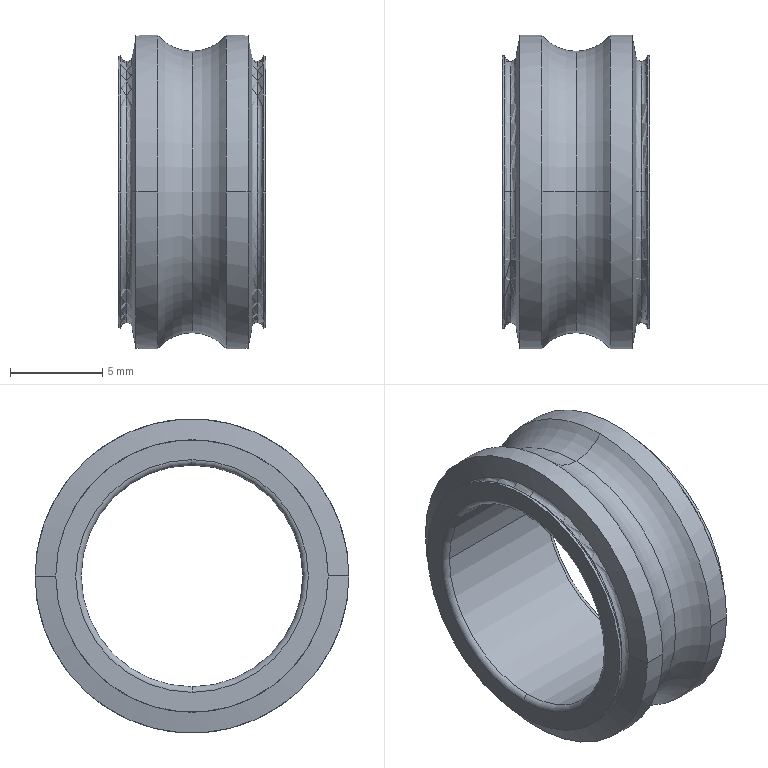Part | SolidWorks | features BaseBody 1 | 1 solid | 32 faces | box 8 x 17 x 17 mm | volume 683.161 mm3 | torus 16 | cylinder 10 | cone 4 | plane 2 | commonest cylinder face diameters 14.75 x4 17 x4 12 x2
STEP:
#1=CARTESIAN_POINT('',(5.849,8.5,0.));
#2=VERTEX_POINT('',#1);
#3=CARTESIAN_POINT('',(7.037,8.5,0.));
#4=VERTEX_POINT('',#3);
#5=CARTESIAN_POINT('',(6.443,8.5,0.));
#6=DIRECTION('',(1.,0.,0.));
#7=VECTOR('',#6,1000.);
#8=LINE('',#5,#7);
#9=EDGE_CURVE('',#2,#4,#8,.T.);
#10=ORIENTED_EDGE('',*,*,#9,.T.);
#11=CARTESIAN_POINT('',(7.037,-8.5,0.));
#12=VERTEX_POINT('',#11);
#13=CARTESIAN_POINT('',(7.037,0.,0.));
#14=DIRECTION('',(1.,0.,0.));
#15=DIRECTION('',(0.,1.,0.));
#16=AXIS2_PLACEMENT_3D('',#13,#14,#15);
#17=CIRCLE('',#16,8.5);
#18=EDGE_CURVE('',#12,#4,#17,.T.);
#19=ORIENTED_EDGE('',*,*,#18,.F.);
#20=CARTESIAN_POINT('',(5.849,-8.5,0.));
#21=VERTEX_POINT('',#20);
#22=CARTESIAN_POINT('',(6.443,-8.5,0.));
#23=DIRECTION('',(-1.,0.,0.));
#24=VECTOR('',#23,1000.);
#25=LINE('',#22,#24);
#26=EDGE_CURVE('',#12,#21,#25,.T.);
#27=ORIENTED_EDGE('',*,*,#26,.T.);
#28=CARTESIAN_POINT('',(5.849,0.,-8.5));
#29=VERTEX_POINT('',#28);
#30=CARTESIAN_POINT('',(5.849,0.,0.));
#31=DIRECTION('',(1.,0.,0.));
#32=DIRECTION('',(0.,1.,0.));
#33=AXIS2_PLACEMENT_3D('',#30,#31,#32);
#34=CIRCLE('',#33,8.5);
#35=EDGE_CURVE('',#21,#29,#34,.T.);
#36=ORIENTED_EDGE('',*,*,#35,.T.);
#37=CARTESIAN_POINT('',(5.849,0.,0.));
#38=DIRECTION('',(1.,0.,0.));
#39=DIRECTION('',(0.,1.,0.));
#40=AXIS2_PLACEMENT_3D('',#37,#38,#39);
#41=CIRCLE('',#40,8.5);
#42=EDGE_CURVE('',#29,#2,#41,.T.);
#43=ORIENTED_EDGE('',*,*,#42,.T.);
#44=EDGE_LOOP('',(#10,#19,#27,#36,#43));
#45=FACE_OUTER_BOUND('',#44,.T.);
#46=CARTESIAN_POINT('',(6.443,0.,0.));
#47=DIRECTION('',(1.,0.,0.));
#48=DIRECTION('',(0.,1.,0.));
#49=AXIS2_PLACEMENT_3D('',#46,#47,#48);
#50=CYLINDRICAL_SURFACE('',#49,8.5);
#51=ADVANCED_FACE('',(#45),#50,.T.);
#52=CARTESIAN_POINT('',(4.,0.,7.619));
#53=VERTEX_POINT('',#52);
#54=CARTESIAN_POINT('',(4.,0.,-7.619));
#55=VERTEX_POINT('',#54);
#56=CARTESIAN_POINT('',(4.,0.,0.));
#57=DIRECTION('',(-1.,0.,0.));
#58=DIRECTION('',(0.,0.,1.));
#59=AXIS2_PLACEMENT_3D('',#56,#57,#58);
#60=CIRCLE('',#59,7.619);
#61=EDGE_CURVE('',#53,#55,#60,.T.);
#62=ORIENTED_EDGE('',*,*,#61,.T.);
#63=CARTESIAN_POINT('',(2.151,0.,-8.5));
#64=VERTEX_POINT('',#63);
#65=CARTESIAN_POINT('',(4.,0.,-10.));
#66=DIRECTION('',(0.,-1.,0.));
#67=DIRECTION('',(0.,0.,-1.));
#68=AXIS2_PLACEMENT_3D('',#65,#66,#67);
#69=CIRCLE('',#68,2.381);
#70=EDGE_CURVE('',#55,#64,#69,.T.);
#71=ORIENTED_EDGE('',*,*,#70,.T.);
#72=CARTESIAN_POINT('',(2.151,8.5,0.));
#73=VERTEX_POINT('',#72);
#74=CARTESIAN_POINT('',(2.151,0.,0.));
#75=DIRECTION('',(1.,0.,0.));
#76=DIRECTION('',(0.,1.,0.));
#77=AXIS2_PLACEMENT_3D('',#74,#75,#76);
#78=CIRCLE('',#77,8.5);
#79=EDGE_CURVE('',#64,#73,#78,.T.);
#80=ORIENTED_EDGE('',*,*,#79,.T.);
#81=CARTESIAN_POINT('',(2.151,0.,8.5));
#82=VERTEX_POINT('',#81);
#83=CARTESIAN_POINT('',(2.151,0.,0.));
#84=DIRECTION('',(1.,0.,0.));
#85=DIRECTION('',(0.,1.,0.));
#86=AXIS2_PLACEMENT_3D('',#83,#84,#85);
#87=CIRCLE('',#86,8.5);
#88=EDGE_CURVE('',#73,#82,#87,.T.);
#89=ORIENTED_EDGE('',*,*,#88,.T.);
#90=CARTESIAN_POINT('',(4.,0.,10.));
#91=DIRECTION('',(0.,-1.,0.));
#92=DIRECTION('',(0.,0.,1.));
#93=AXIS2_PLACEMENT_3D('',#90,#91,#92);
#94=CIRCLE('',#93,2.381);
#95=EDGE_CURVE('',#82,#53,#94,.T.);
#96=ORIENTED_EDGE('',*,*,#95,.T.);
#97=EDGE_LOOP('',(#62,#71,#80,#89,#96));
#98=FACE_OUTER_BOUND('',#97,.T.);
#99=CARTESIAN_POINT('',(4.,0.,0.));
#100=DIRECTION('',(1.,0.,0.));
#101=DIRECTION('',(0.,0.,-1.));
#102=AXIS2_PLACEMENT_3D('',#99,#100,#101);
#103=TOROIDAL_SURFACE('',#102,10.,2.381);
#104=ADVANCED_FACE('',(#98),#103,.F.);
#105=CARTESIAN_POINT('',(0.9631,8.5,0.));
#106=VERTEX_POINT('',#105);
#107=CARTESIAN_POINT('',(1.557,8.5,0.));
#108=DIRECTION('',(1.,0.,0.));
#109=VECTOR('',#108,1000.);
#110=LINE('',#107,#109);
#111=EDGE_CURVE('',#106,#73,#110,.T.);
#112=ORIENTED_EDGE('',*,*,#111,.T.);
#113=ORIENTED_EDGE('',*,*,#79,.F.);
#114=CARTESIAN_POINT('',(2.151,-8.5,0.));
#115=VERTEX_POINT('',#114);
#116=CARTESIAN_POINT('',(2.151,0.,0.));
#117=DIRECTION('',(1.,0.,0.));
#118=DIRECTION('',(0.,1.,0.));
#119=AXIS2_PLACEMENT_3D('',#116,#117,#118);
#120=CIRCLE('',#119,8.5);
#121=EDGE_CURVE('',#115,#64,#120,.T.);
#122=ORIENTED_EDGE('',*,*,#121,.F.);
#123=CARTESIAN_POINT('',(0.9631,-8.5,0.));
#124=VERTEX_POINT('',#123);
#125=CARTESIAN_POINT('',(1.557,-8.5,0.));
#126=DIRECTION('',(-1.,0.,0.));
#127=VECTOR('',#126,1000.);
#128=LINE('',#125,#127);
#129=EDGE_CURVE('',#115,#124,#128,.T.);
#130=ORIENTED_EDGE('',*,*,#129,.T.);
#131=CARTESIAN_POINT('',(0.9631,0.,0.));
#132=DIRECTION('',(1.,0.,0.));
#133=DIRECTION('',(0.,1.,0.));
#134=AXIS2_PLACEMENT_3D('',#131,#132,#133);
#135=CIRCLE('',#134,8.5);
#136=EDGE_CURVE('',#124,#106,#135,.T.);
#137=ORIENTED_EDGE('',*,*,#136,.T.);
#138=EDGE_LOOP('',(#112,#113,#122,#130,#137));
#139=FACE_OUTER_BOUND('',#138,.T.);
#140=CARTESIAN_POINT('',(1.557,0.,0.));
#141=DIRECTION('',(1.,0.,0.));
#142=DIRECTION('',(0.,1.,0.));
#143=AXIS2_PLACEMENT_3D('',#140,#141,#142);
#144=CYLINDRICAL_SURFACE('',#143,8.5);
#145=ADVANCED_FACE('',(#139),#144,.T.);
#146=CARTESIAN_POINT('',(0.7554,7.322,0.));
#147=VERTEX_POINT('',#146);
#148=CARTESIAN_POINT('',(0.8592,7.911,0.));
#149=DIRECTION('',(0.1736,0.9848,0.));
#150=VECTOR('',#149,1000.);
#151=LINE('',#148,#150);
#152=EDGE_CURVE('',#147,#106,#151,.T.);
#153=ORIENTED_EDGE('',*,*,#152,.T.);
#154=ORIENTED_EDGE('',*,*,#136,.F.);
#155=CARTESIAN_POINT('',(0.7554,-7.322,0.));
#156=VERTEX_POINT('',#155);
#157=CARTESIAN_POINT('',(0.8592,-7.911,0.));
#158=DIRECTION('',(-0.1736,0.9848,0.));
#159=VECTOR('',#158,1000.);
#160=LINE('',#157,#159);
#161=EDGE_CURVE('',#124,#156,#160,.T.);
#162=ORIENTED_EDGE('',*,*,#161,.T.);
#163=CARTESIAN_POINT('',(0.7554,0.,-7.322));
#164=VERTEX_POINT('',#163);
#165=CARTESIAN_POINT('',(0.7554,0.,0.));
#166=DIRECTION('',(1.,0.,0.));
#167=DIRECTION('',(0.,1.,0.));
#168=AXIS2_PLACEMENT_3D('',#165,#166,#167);
#169=CIRCLE('',#168,7.322);
#170=EDGE_CURVE('',#156,#164,#169,.T.);
#171=ORIENTED_EDGE('',*,*,#170,.T.);
#172=CARTESIAN_POINT('',(0.7554,0.,0.));
#173=DIRECTION('',(1.,0.,0.));
#174=DIRECTION('',(0.,1.,0.));
#175=AXIS2_PLACEMENT_3D('',#172,#173,#174);
#176=CIRCLE('',#175,7.322);
#177=EDGE_CURVE('',#164,#147,#176,.T.);
#178=ORIENTED_EDGE('',*,*,#177,.T.);
#179=EDGE_LOOP('',(#153,#154,#162,#171,#178));
#180=FACE_OUTER_BOUND('',#179,.T.);
#181=CARTESIAN_POINT('',(0.8592,0.,0.));
#182=DIRECTION('',(1.,0.,0.));
#183=DIRECTION('',(0.,1.,0.));
#184=AXIS2_PLACEMENT_3D('',#181,#182,#183);
#185=CONICAL_SURFACE('',#184,7.911,1.396);
#186=ADVANCED_FACE('',(#180),#185,.T.);
#187=CARTESIAN_POINT('',(0.456,0.,7.071));
#188=VERTEX_POINT('',#187);
#189=CARTESIAN_POINT('',(0.456,0.,-7.071));
#190=VERTEX_POINT('',#189);
#191=CARTESIAN_POINT('',(0.456,0.,0.));
#192=DIRECTION('',(-1.,0.,0.));
#193=DIRECTION('',(0.,0.,1.));
#194=AXIS2_PLACEMENT_3D('',#191,#192,#193);
#195=CIRCLE('',#194,7.071);
#196=EDGE_CURVE('',#188,#190,#195,.T.);
#197=ORIENTED_EDGE('',*,*,#196,.T.);
#198=CARTESIAN_POINT('',(0.152,0.,-7.375));
#199=VERTEX_POINT('',#198);
#200=CARTESIAN_POINT('',(0.456,0.,-7.375));
#201=DIRECTION('',(0.,-1.,0.));
#202=DIRECTION('',(0.,0.,-1.));
#203=AXIS2_PLACEMENT_3D('',#200,#201,#202);
#204=CIRCLE('',#203,0.304);
#205=EDGE_CURVE('',#190,#199,#204,.T.);
#206=ORIENTED_EDGE('',*,*,#205,.T.);
#207=CARTESIAN_POINT('',(0.152,7.375,0.));
#208=VERTEX_POINT('',#207);
#209=CARTESIAN_POINT('',(0.152,0.,0.));
#210=DIRECTION('',(1.,0.,0.));
#211=DIRECTION('',(0.,1.,0.));
#212=AXIS2_PLACEMENT_3D('',#209,#210,#211);
#213=CIRCLE('',#212,7.375);
#214=EDGE_CURVE('',#199,#208,#213,.T.);
#215=ORIENTED_EDGE('',*,*,#214,.T.);
#216=CARTESIAN_POINT('',(0.152,0.,7.375));
#217=VERTEX_POINT('',#216);
#218=CARTESIAN_POINT('',(0.152,0.,0.));
#219=DIRECTION('',(1.,0.,0.));
#220=DIRECTION('',(0.,1.,0.));
#221=AXIS2_PLACEMENT_3D('',#218,#219,#220);
#222=CIRCLE('',#221,7.375);
#223=EDGE_CURVE('',#208,#217,#222,.T.);
#224=ORIENTED_EDGE('',*,*,#223,.T.);
#225=CARTESIAN_POINT('',(0.456,0.,7.375));
#226=DIRECTION('',(0.,-1.,0.));
#227=DIRECTION('',(0.,0.,1.));
#228=AXIS2_PLACEMENT_3D('',#225,#226,#227);
#229=CIRCLE('',#228,0.304);
#230=EDGE_CURVE('',#217,#188,#229,.T.);
#231=ORIENTED_EDGE('',*,*,#230,.T.);
#232=EDGE_LOOP('',(#197,#206,#215,#224,#231));
#233=FACE_OUTER_BOUND('',#232,.T.);
#234=CARTESIAN_POINT('',(0.456,0.,0.));
#235=DIRECTION('',(1.,0.,0.));
#236=DIRECTION('',(0.,0.,-1.));
#237=AXIS2_PLACEMENT_3D('',#234,#235,#236);
#238=TOROIDAL_SURFACE('',#237,7.375,0.304);
#239=ADVANCED_FACE('',(#233),#238,.F.);
#240=CARTESIAN_POINT('',(0.,7.375,0.));
#241=VERTEX_POINT('',#240);
#242=CARTESIAN_POINT('',(0.076,7.375,0.));
#243=DIRECTION('',(1.,0.,0.));
#244=VECTOR('',#243,1000.);
#245=LINE('',#242,#244);
#246=EDGE_CURVE('',#241,#208,#245,.T.);
#247=ORIENTED_EDGE('',*,*,#246,.T.);
#248=ORIENTED_EDGE('',*,*,#214,.F.);
#249=CARTESIAN_POINT('',(0.152,-7.375,0.));
#250=VERTEX_POINT('',#249);
#251=CARTESIAN_POINT('',(0.152,0.,0.));
#252=DIRECTION('',(1.,0.,0.));
#253=DIRECTION('',(0.,1.,0.));
#254=AXIS2_PLACEMENT_3D('',#251,#252,#253);
#255=CIRCLE('',#254,7.375);
#256=EDGE_CURVE('',#250,#199,#255,.T.);
#257=ORIENTED_EDGE('',*,*,#256,.F.);
#258=CARTESIAN_POINT('',(0.,-7.375,0.));
#259=VERTEX_POINT('',#258);
#260=CARTESIAN_POINT('',(0.076,-7.375,0.));
#261=DIRECTION('',(-1.,0.,0.));
#262=VECTOR('',#261,1000.);
#263=LINE('',#260,#262);
#264=EDGE_CURVE('',#250,#259,#263,.T.);
#265=ORIENTED_EDGE('',*,*,#264,.T.);
#266=CARTESIAN_POINT('',(0.,0.,0.));
#267=DIRECTION('',(1.,0.,0.));
#268=DIRECTION('',(0.,1.,0.));
#269=AXIS2_PLACEMENT_3D('',#266,#267,#268);
#270=CIRCLE('',#269,7.375);
#271=EDGE_CURVE('',#259,#241,#270,.T.);
#272=ORIENTED_EDGE('',*,*,#271,.T.);
#273=EDGE_LOOP('',(#247,#248,#257,#265,#272));
#274=FACE_OUTER_BOUND('',#273,.T.);
#275=CARTESIAN_POINT('',(0.076,0.,0.));
#276=DIRECTION('',(1.,0.,0.));
#277=DIRECTION('',(0.,1.,0.));
#278=AXIS2_PLACEMENT_3D('',#275,#276,#277);
#279=CYLINDRICAL_SURFACE('',#278,7.375);
#280=ADVANCED_FACE('',(#274),#279,.T.);
#281=CARTESIAN_POINT('',(0.,0.,6.3));
#282=VERTEX_POINT('',#281);
#283=CARTESIAN_POINT('',(0.,0.,-6.3));
#284=VERTEX_POINT('',#283);
#285=CARTESIAN_POINT('',(0.,0.,0.));
#286=DIRECTION('',(1.,0.,0.));
#287=DIRECTION('',(0.,1.,0.));
#288=AXIS2_PLACEMENT_3D('',#285,#286,#287);
#289=CIRCLE('',#288,6.3);
#290=EDGE_CURVE('',#282,#284,#289,.T.);
#291=ORIENTED_EDGE('',*,*,#290,.T.);
#292=CARTESIAN_POINT('',(0.,0.,0.));
#293=DIRECTION('',(1.,0.,0.));
#294=DIRECTION('',(0.,1.,0.));
#295=AXIS2_PLACEMENT_3D('',#292,#293,#294);
#296=CIRCLE('',#295,6.3);
#297=EDGE_CURVE('',#284,#282,#296,.T.);
#298=ORIENTED_EDGE('',*,*,#297,.T.);
#299=EDGE_LOOP('',(#291,#298));
#300=FACE_BOUND('',#299,.T.);
#301=CARTESIAN_POINT('',(0.,0.,0.));
#302=DIRECTION('',(1.,0.,0.));
#303=DIRECTION('',(0.,1.,0.));
#304=AXIS2_PLACEMENT_3D('',#301,#302,#303);
#305=CIRCLE('',#304,7.375);
#306=EDGE_CURVE('',#241,#259,#305,.T.);
#307=ORIENTED_EDGE('',*,*,#306,.F.);
#308=ORIENTED_EDGE('',*,*,#271,.F.);
#309=EDGE_LOOP('',(#307,#308));
#310=FACE_OUTER_BOUND('',#309,.T.);
#311=CARTESIAN_POINT('',(0.,6.837,0.));
#312=DIRECTION('',(-1.,0.,0.));
#313=DIRECTION('',(0.,0.,1.));
#314=AXIS2_PLACEMENT_3D('',#311,#312,#313);
#315=PLANE('',#314);
#316=ADVANCED_FACE('',(#300,#310),#315,.T.);
#317=CARTESIAN_POINT('',(0.3,0.,-6.));
#318=VERTEX_POINT('',#317);
#319=CARTESIAN_POINT('',(0.3,0.,-6.3));
#320=DIRECTION('',(0.,-1.,0.));
#321=DIRECTION('',(0.,0.,-1.));
#322=AXIS2_PLACEMENT_3D('',#319,#320,#321);
#323=CIRCLE('',#322,0.3);
#324=EDGE_CURVE('',#318,#284,#323,.T.);
#325=ORIENTED_EDGE('',*,*,#324,.T.);
#326=ORIENTED_EDGE('',*,*,#290,.F.);
#327=CARTESIAN_POINT('',(0.3,0.,6.));
#328=VERTEX_POINT('',#327);
#329=CARTESIAN_POINT('',(0.3,0.,6.3));
#330=DIRECTION('',(0.,-1.,0.));
#331=DIRECTION('',(0.,0.,1.));
#332=AXIS2_PLACEMENT_3D('',#329,#330,#331);
#333=CIRCLE('',#332,0.3);
#334=EDGE_CURVE('',#282,#328,#333,.T.);
#335=ORIENTED_EDGE('',*,*,#334,.T.);
#336=CARTESIAN_POINT('',(0.3,-6.,0.));
#337=VERTEX_POINT('',#336);
#338=CARTESIAN_POINT('',(0.3,0.,0.));
#339=DIRECTION('',(1.,0.,0.));
#340=DIRECTION('',(0.,1.,0.));
#341=AXIS2_PLACEMENT_3D('',#338,#339,#340);
#342=CIRCLE('',#341,6.);
#343=EDGE_CURVE('',#328,#337,#342,.T.);
#344=ORIENTED_EDGE('',*,*,#343,.T.);
#345=CARTESIAN_POINT('',(0.3,0.,0.));
#346=DIRECTION('',(1.,0.,0.));
#347=DIRECTION('',(0.,1.,0.));
#348=AXIS2_PLACEMENT_3D('',#345,#346,#347);
#349=CIRCLE('',#348,6.);
#350=EDGE_CURVE('',#337,#318,#349,.T.);
#351=ORIENTED_EDGE('',*,*,#350,.T.);
#352=EDGE_LOOP('',(#325,#326,#335,#344,#351));
#353=FACE_OUTER_BOUND('',#352,.T.);
#354=CARTESIAN_POINT('',(0.3,0.,0.));
#355=DIRECTION('',(1.,0.,0.));
#356=DIRECTION('',(0.,0.,-1.));
#357=AXIS2_PLACEMENT_3D('',#354,#355,#356);
#358=TOROIDAL_SURFACE('',#357,6.3,0.3);
#359=ADVANCED_FACE('',(#353),#358,.T.);
#360=CARTESIAN_POINT('',(0.3,6.,0.));
#361=VERTEX_POINT('',#360);
#362=CARTESIAN_POINT('',(7.7,6.,0.));
#363=VERTEX_POINT('',#362);
#364=CARTESIAN_POINT('',(4.,6.,0.));
#365=DIRECTION('',(1.,0.,0.));
#366=VECTOR('',#365,1000.);
#367=LINE('',#364,#366);
#368=EDGE_CURVE('',#361,#363,#367,.T.);
#369=ORIENTED_EDGE('',*,*,#368,.T.);
#370=CARTESIAN_POINT('',(7.7,0.,6.));
#371=VERTEX_POINT('',#370);
#372=CARTESIAN_POINT('',(7.7,0.,0.));
#373=DIRECTION('',(1.,0.,0.));
#374=DIRECTION('',(0.,1.,0.));
#375=AXIS2_PLACEMENT_3D('',#372,#373,#374);
#376=CIRCLE('',#375,6.);
#377=EDGE_CURVE('',#363,#371,#376,.T.);
#378=ORIENTED_EDGE('',*,*,#377,.T.);
#379=CARTESIAN_POINT('',(7.7,-6.,0.));
#380=VERTEX_POINT('',#379);
#381=CARTESIAN_POINT('',(7.7,0.,0.));
#382=DIRECTION('',(1.,0.,0.));
#383=DIRECTION('',(0.,1.,0.));
#384=AXIS2_PLACEMENT_3D('',#381,#382,#383);
#385=CIRCLE('',#384,6.);
#386=EDGE_CURVE('',#371,#380,#385,.T.);
#387=ORIENTED_EDGE('',*,*,#386,.T.);
#388=CARTESIAN_POINT('',(4.,-6.,0.));
#389=DIRECTION('',(-1.,0.,0.));
#390=VECTOR('',#389,1000.);
#391=LINE('',#388,#390);
#392=EDGE_CURVE('',#380,#337,#391,.T.);
#393=ORIENTED_EDGE('',*,*,#392,.T.);
#394=ORIENTED_EDGE('',*,*,#343,.F.);
#395=CARTESIAN_POINT('',(0.3,0.,0.));
#396=DIRECTION('',(1.,0.,0.));
#397=DIRECTION('',(0.,1.,0.));
#398=AXIS2_PLACEMENT_3D('',#395,#396,#397);
#399=CIRCLE('',#398,6.);
#400=EDGE_CURVE('',#361,#328,#399,.T.);
#401=ORIENTED_EDGE('',*,*,#400,.F.);
#402=EDGE_LOOP('',(#369,#378,#387,#393,#394,#401));
#403=FACE_OUTER_BOUND('',#402,.T.);
#404=CARTESIAN_POINT('',(4.,0.,0.));
#405=DIRECTION('',(1.,0.,0.));
#406=DIRECTION('',(0.,1.,0.));
#407=AXIS2_PLACEMENT_3D('',#404,#405,#406);
#408=CYLINDRICAL_SURFACE('',#407,6.);
#409=ADVANCED_FACE('',(#403),#408,.F.);
#410=CARTESIAN_POINT('',(8.,0.,-6.3));
#411=VERTEX_POINT('',#410);
#412=CARTESIAN_POINT('',(7.7,0.,-6.));
#413=VERTEX_POINT('',#412);
#414=CARTESIAN_POINT('',(7.7,0.,-6.3));
#415=DIRECTION('',(0.,-1.,0.));
#416=DIRECTION('',(0.,0.,-1.));
#417=AXIS2_PLACEMENT_3D('',#414,#415,#416);
#418=CIRCLE('',#417,0.3);
#419=EDGE_CURVE('',#411,#413,#418,.T.);
#420=ORIENTED_EDGE('',*,*,#419,.T.);
#421=CARTESIAN_POINT('',(7.7,0.,0.));
#422=DIRECTION('',(1.,0.,0.));
#423=DIRECTION('',(0.,1.,0.));
#424=AXIS2_PLACEMENT_3D('',#421,#422,#423);
#425=CIRCLE('',#424,6.);
#426=EDGE_CURVE('',#380,#413,#425,.T.);
#427=ORIENTED_EDGE('',*,*,#426,.F.);
#428=ORIENTED_EDGE('',*,*,#386,.F.);
#429=CARTESIAN_POINT('',(8.,0.,6.3));
#430=VERTEX_POINT('',#429);
#431=CARTESIAN_POINT('',(7.7,0.,6.3));
#432=DIRECTION('',(0.,-1.,0.));
#433=DIRECTION('',(0.,0.,1.));
#434=AXIS2_PLACEMENT_3D('',#431,#432,#433);
#435=CIRCLE('',#434,0.3);
#436=EDGE_CURVE('',#371,#430,#435,.T.);
#437=ORIENTED_EDGE('',*,*,#436,.T.);
#438=CARTESIAN_POINT('',(8.,0.,0.));
#439=DIRECTION('',(1.,0.,0.));
#440=DIRECTION('',(0.,1.,0.));
#441=AXIS2_PLACEMENT_3D('',#438,#439,#440);
#442=CIRCLE('',#441,6.3);
#443=EDGE_CURVE('',#430,#411,#442,.T.);
#444=ORIENTED_EDGE('',*,*,#443,.T.);
#445=EDGE_LOOP('',(#420,#427,#428,#437,#444));
#446=FACE_OUTER_BOUND('',#445,.T.);
#447=CARTESIAN_POINT('',(7.7,0.,0.));
#448=DIRECTION('',(1.,0.,0.));
#449=DIRECTION('',(0.,0.,-1.));
#450=AXIS2_PLACEMENT_3D('',#447,#448,#449);
#451=TOROIDAL_SURFACE('',#450,6.3,0.3);
#452=ADVANCED_FACE('',(#446),#451,.T.);
#453=CARTESIAN_POINT('',(8.,0.,0.));
#454=DIRECTION('',(1.,0.,0.));
#455=DIRECTION('',(0.,1.,0.));
#456=AXIS2_PLACEMENT_3D('',#453,#454,#455);
#457=CIRCLE('',#456,6.3);
#458=EDGE_CURVE('',#411,#430,#457,.T.);
#459=ORIENTED_EDGE('',*,*,#458,.F.);
#460=ORIENTED_EDGE('',*,*,#443,.F.);
#461=EDGE_LOOP('',(#459,#460));
#462=FACE_BOUND('',#461,.T.);
#463=CARTESIAN_POINT('',(8.,7.375,0.));
#464=VERTEX_POINT('',#463);
#465=CARTESIAN_POINT('',(8.,-7.375,0.));
#466=VERTEX_POINT('',#465);
#467=CARTESIAN_POINT('',(8.,0.,0.));
#468=DIRECTION('',(1.,0.,0.));
#469=DIRECTION('',(0.,1.,0.));
#470=AXIS2_PLACEMENT_3D('',#467,#468,#469);
#471=CIRCLE('',#470,7.375);
#472=EDGE_CURVE('',#464,#466,#471,.T.);
#473=ORIENTED_EDGE('',*,*,#472,.T.);
#474=CARTESIAN_POINT('',(8.,0.,0.));
#475=DIRECTION('',(1.,0.,0.));
#476=DIRECTION('',(0.,1.,0.));
#477=AXIS2_PLACEMENT_3D('',#474,#475,#476);
#478=CIRCLE('',#477,7.375);
#479=EDGE_CURVE('',#466,#464,#478,.T.);
#480=ORIENTED_EDGE('',*,*,#479,.T.);
#481=EDGE_LOOP('',(#473,#480));
#482=FACE_OUTER_BOUND('',#481,.T.);
#483=CARTESIAN_POINT('',(8.,6.837,0.));
#484=DIRECTION('',(1.,0.,0.));
#485=DIRECTION('',(0.,1.,0.));
#486=AXIS2_PLACEMENT_3D('',#483,#484,#485);
#487=PLANE('',#486);
#488=ADVANCED_FACE('',(#462,#482),#487,.T.);
#489=CARTESIAN_POINT('',(7.848,7.375,0.));
#490=VERTEX_POINT('',#489);
#491=CARTESIAN_POINT('',(7.924,7.375,0.));
#492=DIRECTION('',(1.,0.,0.));
#493=VECTOR('',#492,1000.);
#494=LINE('',#491,#493);
#495=EDGE_CURVE('',#490,#464,#494,.T.);
#496=ORIENTED_EDGE('',*,*,#495,.T.);
#497=ORIENTED_EDGE('',*,*,#479,.F.);
#498=CARTESIAN_POINT('',(7.848,-7.375,0.));
#499=VERTEX_POINT('',#498);
#500=CARTESIAN_POINT('',(7.924,-7.375,0.));
#501=DIRECTION('',(-1.,0.,0.));
#502=VECTOR('',#501,1000.);
#503=LINE('',#500,#502);
#504=EDGE_CURVE('',#466,#499,#503,.T.);
#505=ORIENTED_EDGE('',*,*,#504,.T.);
#506=CARTESIAN_POINT('',(7.848,0.,-7.375));
#507=VERTEX_POINT('',#506);
#508=CARTESIAN_POINT('',(7.848,0.,0.));
#509=DIRECTION('',(1.,0.,0.));
#510=DIRECTION('',(0.,1.,0.));
#511=AXIS2_PLACEMENT_3D('',#508,#509,#510);
#512=CIRCLE('',#511,7.375);
#513=EDGE_CURVE('',#499,#507,#512,.T.);
#514=ORIENTED_EDGE('',*,*,#513,.T.);
#515=CARTESIAN_POINT('',(7.848,0.,0.));
#516=DIRECTION('',(1.,0.,0.));
#517=DIRECTION('',(0.,1.,0.));
#518=AXIS2_PLACEMENT_3D('',#515,#516,#517);
#519=CIRCLE('',#518,7.375);
#520=EDGE_CURVE('',#507,#490,#519,.T.);
#521=ORIENTED_EDGE('',*,*,#520,.T.);
#522=EDGE_LOOP('',(#496,#497,#505,#514,#521));
#523=FACE_OUTER_BOUND('',#522,.T.);
#524=CARTESIAN_POINT('',(7.924,0.,0.));
#525=DIRECTION('',(1.,0.,0.));
#526=DIRECTION('',(0.,1.,0.));
#527=AXIS2_PLACEMENT_3D('',#524,#525,#526);
#528=CYLINDRICAL_SURFACE('',#527,7.375);
#529=ADVANCED_FACE('',(#523),#528,.T.);
#530=CARTESIAN_POINT('',(7.544,0.,7.071));
#531=VERTEX_POINT('',#530);
#532=CARTESIAN_POINT('',(7.544,0.,-7.071));
#533=VERTEX_POINT('',#532);
#534=CARTESIAN_POINT('',(7.544,0.,0.));
#535=DIRECTION('',(-1.,0.,0.));
#536=DIRECTION('',(0.,0.,1.));
#537=AXIS2_PLACEMENT_3D('',#534,#535,#536);
#538=CIRCLE('',#537,7.071);
#539=EDGE_CURVE('',#531,#533,#538,.T.);
#540=ORIENTED_EDGE('',*,*,#539,.T.);
#541=CARTESIAN_POINT('',(7.245,0.,-7.322));
#542=VERTEX_POINT('',#541);
#543=CARTESIAN_POINT('',(7.544,0.,-7.375));
#544=DIRECTION('',(0.,-1.,0.));
#545=DIRECTION('',(0.,0.,-1.));
#546=AXIS2_PLACEMENT_3D('',#543,#544,#545);
#547=CIRCLE('',#546,0.304);
#548=EDGE_CURVE('',#533,#542,#547,.T.);
#549=ORIENTED_EDGE('',*,*,#548,.T.);
#550=CARTESIAN_POINT('',(7.245,7.322,0.));
#551=VERTEX_POINT('',#550);
#552=CARTESIAN_POINT('',(7.245,0.,0.));
#553=DIRECTION('',(1.,0.,0.));
#554=DIRECTION('',(0.,1.,0.));
#555=AXIS2_PLACEMENT_3D('',#552,#553,#554);
#556=CIRCLE('',#555,7.322);
#557=EDGE_CURVE('',#542,#551,#556,.T.);
#558=ORIENTED_EDGE('',*,*,#557,.T.);
#559=CARTESIAN_POINT('',(7.245,0.,7.322));
#560=VERTEX_POINT('',#559);
#561=CARTESIAN_POINT('',(7.245,0.,0.));
#562=DIRECTION('',(1.,0.,0.));
#563=DIRECTION('',(0.,1.,0.));
#564=AXIS2_PLACEMENT_3D('',#561,#562,#563);
#565=CIRCLE('',#564,7.322);
#566=EDGE_CURVE('',#551,#560,#565,.T.);
#567=ORIENTED_EDGE('',*,*,#566,.T.);
#568=CARTESIAN_POINT('',(7.544,0.,7.375));
#569=DIRECTION('',(0.,-1.,0.));
#570=DIRECTION('',(0.,0.,1.));
#571=AXIS2_PLACEMENT_3D('',#568,#569,#570);
#572=CIRCLE('',#571,0.304);
#573=EDGE_CURVE('',#560,#531,#572,.T.);
#574=ORIENTED_EDGE('',*,*,#573,.T.);
#575=EDGE_LOOP('',(#540,#549,#558,#567,#574));
#576=FACE_OUTER_BOUND('',#575,.T.);
#577=CARTESIAN_POINT('',(7.544,0.,0.));
#578=DIRECTION('',(1.,0.,0.));
#579=DIRECTION('',(0.,0.,-1.));
#580=AXIS2_PLACEMENT_3D('',#577,#578,#579);
#581=TOROIDAL_SURFACE('',#580,7.375,0.304);
#582=ADVANCED_FACE('',(#576),#581,.F.);
#583=CARTESIAN_POINT('',(7.141,7.911,0.));
#584=DIRECTION('',(0.1736,-0.9848,0.));
#585=VECTOR('',#584,1000.);
#586=LINE('',#583,#585);
#587=EDGE_CURVE('',#4,#551,#586,.T.);
#588=ORIENTED_EDGE('',*,*,#587,.T.);
#589=ORIENTED_EDGE('',*,*,#557,.F.);
#590=CARTESIAN_POINT('',(7.245,-7.322,0.));
#591=VERTEX_POINT('',#590);
#592=CARTESIAN_POINT('',(7.245,0.,0.));
#593=DIRECTION('',(1.,0.,0.));
#594=DIRECTION('',(0.,1.,0.));
#595=AXIS2_PLACEMENT_3D('',#592,#593,#594);
#596=CIRCLE('',#595,7.322);
#597=EDGE_CURVE('',#591,#542,#596,.T.);
#598=ORIENTED_EDGE('',*,*,#597,.F.);
#599=CARTESIAN_POINT('',(7.141,-7.911,0.));
#600=DIRECTION('',(-0.1736,-0.9848,0.));
#601=VECTOR('',#600,1000.);
#602=LINE('',#599,#601);
#603=EDGE_CURVE('',#591,#12,#602,.T.);
#604=ORIENTED_EDGE('',*,*,#603,.T.);
#605=ORIENTED_EDGE('',*,*,#18,.T.);
#606=EDGE_LOOP('',(#588,#589,#598,#604,#605));
#607=FACE_OUTER_BOUND('',#606,.T.);
#608=CARTESIAN_POINT('',(7.141,0.,0.));
#609=DIRECTION('',(-1.,0.,0.));
#610=DIRECTION('',(0.,1.,0.));
#611=AXIS2_PLACEMENT_3D('',#608,#609,#610);
#612=CONICAL_SURFACE('',#611,7.911,1.396);
#613=ADVANCED_FACE('',(#607),#612,.T.);
#614=ORIENTED_EDGE('',*,*,#587,.F.);
#615=CARTESIAN_POINT('',(7.037,0.,0.));
#616=DIRECTION('',(1.,0.,0.));
#617=DIRECTION('',(0.,1.,0.));
#618=AXIS2_PLACEMENT_3D('',#615,#616,#617);
#619=CIRCLE('',#618,8.5);
#620=EDGE_CURVE('',#4,#12,#619,.T.);
#621=ORIENTED_EDGE('',*,*,#620,.T.);
#622=ORIENTED_EDGE('',*,*,#603,.F.);
#623=CARTESIAN_POINT('',(7.245,0.,0.));
#624=DIRECTION('',(1.,0.,0.));
#625=DIRECTION('',(0.,1.,0.));
#626=AXIS2_PLACEMENT_3D('',#623,#624,#625);
#627=CIRCLE('',#626,7.322);
#628=EDGE_CURVE('',#560,#591,#627,.T.);
#629=ORIENTED_EDGE('',*,*,#628,.F.);
#630=ORIENTED_EDGE('',*,*,#566,.F.);
#631=EDGE_LOOP('',(#614,#621,#622,#629,#630));
#632=FACE_OUTER_BOUND('',#631,.T.);
#633=CARTESIAN_POINT('',(7.141,0.,0.));
#634=DIRECTION('',(-1.,0.,0.));
#635=DIRECTION('',(0.,1.,0.));
#636=AXIS2_PLACEMENT_3D('',#633,#634,#635);
#637=CONICAL_SURFACE('',#636,7.911,1.396);
#638=ADVANCED_FACE('',(#632),#637,.T.);
#639=CARTESIAN_POINT('',(7.544,0.,0.));
#640=DIRECTION('',(-1.,0.,0.));
#641=DIRECTION('',(0.,0.,1.));
#642=AXIS2_PLACEMENT_3D('',#639,#640,#641);
#643=CIRCLE('',#642,7.071);
#644=EDGE_CURVE('',#533,#531,#643,.T.);
#645=ORIENTED_EDGE('',*,*,#644,.T.);
#646=ORIENTED_EDGE('',*,*,#573,.F.);
#647=ORIENTED_EDGE('',*,*,#628,.T.);
#648=ORIENTED_EDGE('',*,*,#597,.T.);
#649=ORIENTED_EDGE('',*,*,#548,.F.);
#650=EDGE_LOOP('',(#645,#646,#647,#648,#649));
#651=FACE_OUTER_BOUND('',#650,.T.);
#652=CARTESIAN_POINT('',(7.544,0.,0.));
#653=DIRECTION('',(1.,0.,0.));
#654=DIRECTION('',(0.,0.,-1.));
#655=AXIS2_PLACEMENT_3D('',#652,#653,#654);
#656=TOROIDAL_SURFACE('',#655,7.375,0.304);
#657=ADVANCED_FACE('',(#651),#656,.F.);
#658=ORIENTED_EDGE('',*,*,#495,.F.);
#659=CARTESIAN_POINT('',(7.848,0.,7.375));
#660=VERTEX_POINT('',#659);
#661=CARTESIAN_POINT('',(7.848,0.,0.));
#662=DIRECTION('',(1.,0.,0.));
#663=DIRECTION('',(0.,1.,0.));
#664=AXIS2_PLACEMENT_3D('',#661,#662,#663);
#665=CIRCLE('',#664,7.375);
#666=EDGE_CURVE('',#490,#660,#665,.T.);
#667=ORIENTED_EDGE('',*,*,#666,.T.);
#668=CARTESIAN_POINT('',(7.848,0.,0.));
#669=DIRECTION('',(1.,0.,0.));
#670=DIRECTION('',(0.,1.,0.));
#671=AXIS2_PLACEMENT_3D('',#668,#669,#670);
#672=CIRCLE('',#671,7.375);
#673=EDGE_CURVE('',#660,#499,#672,.T.);
#674=ORIENTED_EDGE('',*,*,#673,.T.);
#675=ORIENTED_EDGE('',*,*,#504,.F.);
#676=ORIENTED_EDGE('',*,*,#472,.F.);
#677=EDGE_LOOP('',(#658,#667,#674,#675,#676));
#678=FACE_OUTER_BOUND('',#677,.T.);
#679=CARTESIAN_POINT('',(7.924,0.,0.));
#680=DIRECTION('',(1.,0.,0.));
#681=DIRECTION('',(0.,1.,0.));
#682=AXIS2_PLACEMENT_3D('',#679,#680,#681);
#683=CYLINDRICAL_SURFACE('',#682,7.375);
#684=ADVANCED_FACE('',(#678),#683,.T.);
#685=ORIENTED_EDGE('',*,*,#419,.F.);
#686=ORIENTED_EDGE('',*,*,#458,.T.);
#687=ORIENTED_EDGE('',*,*,#436,.F.);
#688=ORIENTED_EDGE('',*,*,#377,.F.);
#689=CARTESIAN_POINT('',(7.7,0.,0.));
#690=DIRECTION('',(1.,0.,0.));
#691=DIRECTION('',(0.,1.,0.));
#692=AXIS2_PLACEMENT_3D('',#689,#690,#691);
#693=CIRCLE('',#692,6.);
#694=EDGE_CURVE('',#413,#363,#693,.T.);
#695=ORIENTED_EDGE('',*,*,#694,.F.);
#696=EDGE_LOOP('',(#685,#686,#687,#688,#695));
#697=FACE_OUTER_BOUND('',#696,.T.);
#698=CARTESIAN_POINT('',(7.7,0.,0.));
#699=DIRECTION('',(1.,0.,0.));
#700=DIRECTION('',(0.,0.,-1.));
#701=AXIS2_PLACEMENT_3D('',#698,#699,#700);
#702=TOROIDAL_SURFACE('',#701,6.3,0.3);
#703=ADVANCED_FACE('',(#697),#702,.T.);
#704=ORIENTED_EDGE('',*,*,#368,.F.);
#705=CARTESIAN_POINT('',(0.3,0.,0.));
#706=DIRECTION('',(1.,0.,0.));
#707=DIRECTION('',(0.,1.,0.));
#708=AXIS2_PLACEMENT_3D('',#705,#706,#707);
#709=CIRCLE('',#708,6.);
#710=EDGE_CURVE('',#318,#361,#709,.T.);
#711=ORIENTED_EDGE('',*,*,#710,.F.);
#712=ORIENTED_EDGE('',*,*,#350,.F.);
#713=ORIENTED_EDGE('',*,*,#392,.F.);
#714=ORIENTED_EDGE('',*,*,#426,.T.);
#715=ORIENTED_EDGE('',*,*,#694,.T.);
#716=EDGE_LOOP('',(#704,#711,#712,#713,#714,#715));
#717=FACE_OUTER_BOUND('',#716,.T.);
#718=CARTESIAN_POINT('',(4.,0.,0.));
#719=DIRECTION('',(1.,0.,0.));
#720=DIRECTION('',(0.,1.,0.));
#721=AXIS2_PLACEMENT_3D('',#718,#719,#720);
#722=CYLINDRICAL_SURFACE('',#721,6.);
#723=ADVANCED_FACE('',(#717),#722,.F.);
#724=ORIENTED_EDGE('',*,*,#324,.F.);
#725=ORIENTED_EDGE('',*,*,#710,.T.);
#726=ORIENTED_EDGE('',*,*,#400,.T.);
#727=ORIENTED_EDGE('',*,*,#334,.F.);
#728=ORIENTED_EDGE('',*,*,#297,.F.);
#729=EDGE_LOOP('',(#724,#725,#726,#727,#728));
#730=FACE_OUTER_BOUND('',#729,.T.);
#731=CARTESIAN_POINT('',(0.3,0.,0.));
#732=DIRECTION('',(1.,0.,0.));
#733=DIRECTION('',(0.,0.,-1.));
#734=AXIS2_PLACEMENT_3D('',#731,#732,#733);
#735=TOROIDAL_SURFACE('',#734,6.3,0.3);
#736=ADVANCED_FACE('',(#730),#735,.T.);
#737=ORIENTED_EDGE('',*,*,#246,.F.);
#738=ORIENTED_EDGE('',*,*,#306,.T.);
#739=ORIENTED_EDGE('',*,*,#264,.F.);
#740=CARTESIAN_POINT('',(0.152,0.,0.));
#741=DIRECTION('',(1.,0.,0.));
#742=DIRECTION('',(0.,1.,0.));
#743=AXIS2_PLACEMENT_3D('',#740,#741,#742);
#744=CIRCLE('',#743,7.375);
#745=EDGE_CURVE('',#217,#250,#744,.T.);
#746=ORIENTED_EDGE('',*,*,#745,.F.);
#747=ORIENTED_EDGE('',*,*,#223,.F.);
#748=EDGE_LOOP('',(#737,#738,#739,#746,#747));
#749=FACE_OUTER_BOUND('',#748,.T.);
#750=CARTESIAN_POINT('',(0.076,0.,0.));
#751=DIRECTION('',(1.,0.,0.));
#752=DIRECTION('',(0.,1.,0.));
#753=AXIS2_PLACEMENT_3D('',#750,#751,#752);
#754=CYLINDRICAL_SURFACE('',#753,7.375);
#755=ADVANCED_FACE('',(#749),#754,.T.);
#756=CARTESIAN_POINT('',(0.456,0.,0.));
#757=DIRECTION('',(-1.,0.,0.));
#758=DIRECTION('',(0.,0.,1.));
#759=AXIS2_PLACEMENT_3D('',#756,#757,#758);
#760=CIRCLE('',#759,7.071);
#761=EDGE_CURVE('',#190,#188,#760,.T.);
#762=ORIENTED_EDGE('',*,*,#761,.T.);
#763=ORIENTED_EDGE('',*,*,#230,.F.);
#764=ORIENTED_EDGE('',*,*,#745,.T.);
#765=ORIENTED_EDGE('',*,*,#256,.T.);
#766=ORIENTED_EDGE('',*,*,#205,.F.);
#767=EDGE_LOOP('',(#762,#763,#764,#765,#766));
#768=FACE_OUTER_BOUND('',#767,.T.);
#769=CARTESIAN_POINT('',(0.456,0.,0.));
#770=DIRECTION('',(1.,0.,0.));
#771=DIRECTION('',(0.,0.,-1.));
#772=AXIS2_PLACEMENT_3D('',#769,#770,#771);
#773=TOROIDAL_SURFACE('',#772,7.375,0.304);
#774=ADVANCED_FACE('',(#768),#773,.F.);
#775=ORIENTED_EDGE('',*,*,#152,.F.);
#776=CARTESIAN_POINT('',(0.7554,0.,7.322));
#777=VERTEX_POINT('',#776);
#778=CARTESIAN_POINT('',(0.7554,0.,0.));
#779=DIRECTION('',(1.,0.,0.));
#780=DIRECTION('',(0.,1.,0.));
#781=AXIS2_PLACEMENT_3D('',#778,#779,#780);
#782=CIRCLE('',#781,7.322);
#783=EDGE_CURVE('',#147,#777,#782,.T.);
#784=ORIENTED_EDGE('',*,*,#783,.T.);
#785=CARTESIAN_POINT('',(0.7554,0.,0.));
#786=DIRECTION('',(1.,0.,0.));
#787=DIRECTION('',(0.,1.,0.));
#788=AXIS2_PLACEMENT_3D('',#785,#786,#787);
#789=CIRCLE('',#788,7.322);
#790=EDGE_CURVE('',#777,#156,#789,.T.);
#791=ORIENTED_EDGE('',*,*,#790,.T.);
#792=ORIENTED_EDGE('',*,*,#161,.F.);
#793=CARTESIAN_POINT('',(0.9631,0.,0.));
#794=DIRECTION('',(1.,0.,0.));
#795=DIRECTION('',(0.,1.,0.));
#796=AXIS2_PLACEMENT_3D('',#793,#794,#795);
#797=CIRCLE('',#796,8.5);
#798=EDGE_CURVE('',#106,#124,#797,.T.);
#799=ORIENTED_EDGE('',*,*,#798,.F.);
#800=EDGE_LOOP('',(#775,#784,#791,#792,#799));
#801=FACE_OUTER_BOUND('',#800,.T.);
#802=CARTESIAN_POINT('',(0.8592,0.,0.));
#803=DIRECTION('',(1.,0.,0.));
#804=DIRECTION('',(0.,1.,0.));
#805=AXIS2_PLACEMENT_3D('',#802,#803,#804);
#806=CONICAL_SURFACE('',#805,7.911,1.396);
#807=ADVANCED_FACE('',(#801),#806,.T.);
#808=ORIENTED_EDGE('',*,*,#111,.F.);
#809=ORIENTED_EDGE('',*,*,#798,.T.);
#810=ORIENTED_EDGE('',*,*,#129,.F.);
#811=CARTESIAN_POINT('',(2.151,0.,0.));
#812=DIRECTION('',(1.,0.,0.));
#813=DIRECTION('',(0.,1.,0.));
#814=AXIS2_PLACEMENT_3D('',#811,#812,#813);
#815=CIRCLE('',#814,8.5);
#816=EDGE_CURVE('',#82,#115,#815,.T.);
#817=ORIENTED_EDGE('',*,*,#816,.F.);
#818=ORIENTED_EDGE('',*,*,#88,.F.);
#819=EDGE_LOOP('',(#808,#809,#810,#817,#818));
#820=FACE_OUTER_BOUND('',#819,.T.);
#821=CARTESIAN_POINT('',(1.557,0.,0.));
#822=DIRECTION('',(1.,0.,0.));
#823=DIRECTION('',(0.,1.,0.));
#824=AXIS2_PLACEMENT_3D('',#821,#822,#823);
#825=CYLINDRICAL_SURFACE('',#824,8.5);
#826=ADVANCED_FACE('',(#820),#825,.T.);
#827=CARTESIAN_POINT('',(4.,0.,0.));
#828=DIRECTION('',(-1.,0.,0.));
#829=DIRECTION('',(0.,0.,1.));
#830=AXIS2_PLACEMENT_3D('',#827,#828,#829);
#831=CIRCLE('',#830,7.619);
#832=EDGE_CURVE('',#55,#53,#831,.T.);
#833=ORIENTED_EDGE('',*,*,#832,.T.);
#834=ORIENTED_EDGE('',*,*,#95,.F.);
#835=ORIENTED_EDGE('',*,*,#816,.T.);
#836=ORIENTED_EDGE('',*,*,#121,.T.);
#837=ORIENTED_EDGE('',*,*,#70,.F.);
#838=EDGE_LOOP('',(#833,#834,#835,#836,#837));
#839=FACE_OUTER_BOUND('',#838,.T.);
#840=CARTESIAN_POINT('',(4.,0.,0.));
#841=DIRECTION('',(1.,0.,0.));
#842=DIRECTION('',(0.,0.,-1.));
#843=AXIS2_PLACEMENT_3D('',#840,#841,#842);
#844=TOROIDAL_SURFACE('',#843,10.,2.381);
#845=ADVANCED_FACE('',(#839),#844,.F.);
#846=ORIENTED_EDGE('',*,*,#9,.F.);
#847=CARTESIAN_POINT('',(5.849,0.,8.5));
#848=VERTEX_POINT('',#847);
#849=CARTESIAN_POINT('',(5.849,0.,0.));
#850=DIRECTION('',(1.,0.,0.));
#851=DIRECTION('',(0.,1.,0.));
#852=AXIS2_PLACEMENT_3D('',#849,#850,#851);
#853=CIRCLE('',#852,8.5);
#854=EDGE_CURVE('',#2,#848,#853,.T.);
#855=ORIENTED_EDGE('',*,*,#854,.T.);
#856=CARTESIAN_POINT('',(5.849,0.,0.));
#857=DIRECTION('',(1.,0.,0.));
#858=DIRECTION('',(0.,1.,0.));
#859=AXIS2_PLACEMENT_3D('',#856,#857,#858);
#860=CIRCLE('',#859,8.5);
#861=EDGE_CURVE('',#848,#21,#860,.T.);
#862=ORIENTED_EDGE('',*,*,#861,.T.);
#863=ORIENTED_EDGE('',*,*,#26,.F.);
#864=ORIENTED_EDGE('',*,*,#620,.F.);
#865=EDGE_LOOP('',(#846,#855,#862,#863,#864));
#866=FACE_OUTER_BOUND('',#865,.T.);
#867=CARTESIAN_POINT('',(6.443,0.,0.));
#868=DIRECTION('',(1.,0.,0.));
#869=DIRECTION('',(0.,1.,0.));
#870=AXIS2_PLACEMENT_3D('',#867,#868,#869);
#871=CYLINDRICAL_SURFACE('',#870,8.5);
#872=ADVANCED_FACE('',(#866),#871,.T.);
#873=ORIENTED_EDGE('',*,*,#832,.F.);
#874=CARTESIAN_POINT('',(4.,0.,-10.));
#875=DIRECTION('',(0.,-1.,0.));
#876=DIRECTION('',(0.,0.,-1.));
#877=AXIS2_PLACEMENT_3D('',#874,#875,#876);
#878=CIRCLE('',#877,2.381);
#879=EDGE_CURVE('',#29,#55,#878,.T.);
#880=ORIENTED_EDGE('',*,*,#879,.F.);
#881=ORIENTED_EDGE('',*,*,#35,.F.);
#882=ORIENTED_EDGE('',*,*,#861,.F.);
#883=CARTESIAN_POINT('',(4.,0.,10.));
#884=DIRECTION('',(0.,-1.,0.));
#885=DIRECTION('',(0.,0.,1.));
#886=AXIS2_PLACEMENT_3D('',#883,#884,#885);
#887=CIRCLE('',#886,2.381);
#888=EDGE_CURVE('',#53,#848,#887,.T.);
#889=ORIENTED_EDGE('',*,*,#888,.F.);
#890=EDGE_LOOP('',(#873,#880,#881,#882,#889));
#891=FACE_OUTER_BOUND('',#890,.T.);
#892=CARTESIAN_POINT('',(4.,0.,0.));
#893=DIRECTION('',(1.,0.,0.));
#894=DIRECTION('',(0.,0.,-1.));
#895=AXIS2_PLACEMENT_3D('',#892,#893,#894);
#896=TOROIDAL_SURFACE('',#895,10.,2.381);
#897=ADVANCED_FACE('',(#891),#896,.F.);
#898=ORIENTED_EDGE('',*,*,#761,.F.);
#899=CARTESIAN_POINT('',(0.456,0.,-7.375));
#900=DIRECTION('',(0.,-1.,0.));
#901=DIRECTION('',(0.,0.,-1.));
#902=AXIS2_PLACEMENT_3D('',#899,#900,#901);
#903=CIRCLE('',#902,0.304);
#904=EDGE_CURVE('',#164,#190,#903,.T.);
#905=ORIENTED_EDGE('',*,*,#904,.F.);
#906=ORIENTED_EDGE('',*,*,#170,.F.);
#907=ORIENTED_EDGE('',*,*,#790,.F.);
#908=CARTESIAN_POINT('',(0.456,0.,7.375));
#909=DIRECTION('',(0.,-1.,0.));
#910=DIRECTION('',(0.,0.,1.));
#911=AXIS2_PLACEMENT_3D('',#908,#909,#910);
#912=CIRCLE('',#911,0.304);
#913=EDGE_CURVE('',#188,#777,#912,.T.);
#914=ORIENTED_EDGE('',*,*,#913,.F.);
#915=EDGE_LOOP('',(#898,#905,#906,#907,#914));
#916=FACE_OUTER_BOUND('',#915,.T.);
#917=CARTESIAN_POINT('',(0.456,0.,0.));
#918=DIRECTION('',(1.,0.,0.));
#919=DIRECTION('',(0.,0.,-1.));
#920=AXIS2_PLACEMENT_3D('',#917,#918,#919);
#921=TOROIDAL_SURFACE('',#920,7.375,0.304);
#922=ADVANCED_FACE('',(#916),#921,.F.);
#923=ORIENTED_EDGE('',*,*,#644,.F.);
#924=CARTESIAN_POINT('',(7.544,0.,-7.375));
#925=DIRECTION('',(0.,-1.,0.));
#926=DIRECTION('',(0.,0.,-1.));
#927=AXIS2_PLACEMENT_3D('',#924,#925,#926);
#928=CIRCLE('',#927,0.304);
#929=EDGE_CURVE('',#507,#533,#928,.T.);
#930=ORIENTED_EDGE('',*,*,#929,.F.);
#931=ORIENTED_EDGE('',*,*,#513,.F.);
#932=ORIENTED_EDGE('',*,*,#673,.F.);
#933=CARTESIAN_POINT('',(7.544,0.,7.375));
#934=DIRECTION('',(0.,-1.,0.));
#935=DIRECTION('',(0.,0.,1.));
#936=AXIS2_PLACEMENT_3D('',#933,#934,#935);
#937=CIRCLE('',#936,0.304);
#938=EDGE_CURVE('',#531,#660,#937,.T.);
#939=ORIENTED_EDGE('',*,*,#938,.F.);
#940=EDGE_LOOP('',(#923,#930,#931,#932,#939));
#941=FACE_OUTER_BOUND('',#940,.T.);
#942=CARTESIAN_POINT('',(7.544,0.,0.));
#943=DIRECTION('',(1.,0.,0.));
#944=DIRECTION('',(0.,0.,-1.));
#945=AXIS2_PLACEMENT_3D('',#942,#943,#944);
#946=TOROIDAL_SURFACE('',#945,7.375,0.304);
#947=ADVANCED_FACE('',(#941),#946,.F.);
#948=ORIENTED_EDGE('',*,*,#539,.F.);
#949=ORIENTED_EDGE('',*,*,#938,.T.);
#950=ORIENTED_EDGE('',*,*,#666,.F.);
#951=ORIENTED_EDGE('',*,*,#520,.F.);
#952=ORIENTED_EDGE('',*,*,#929,.T.);
#953=EDGE_LOOP('',(#948,#949,#950,#951,#952));
#954=FACE_OUTER_BOUND('',#953,.T.);
#955=CARTESIAN_POINT('',(7.544,0.,0.));
#956=DIRECTION('',(1.,0.,0.));
#957=DIRECTION('',(0.,0.,-1.));
#958=AXIS2_PLACEMENT_3D('',#955,#956,#957);
#959=TOROIDAL_SURFACE('',#958,7.375,0.304);
#960=ADVANCED_FACE('',(#954),#959,.F.);
#961=ORIENTED_EDGE('',*,*,#196,.F.);
#962=ORIENTED_EDGE('',*,*,#913,.T.);
#963=ORIENTED_EDGE('',*,*,#783,.F.);
#964=ORIENTED_EDGE('',*,*,#177,.F.);
#965=ORIENTED_EDGE('',*,*,#904,.T.);
#966=EDGE_LOOP('',(#961,#962,#963,#964,#965));
#967=FACE_OUTER_BOUND('',#966,.T.);
#968=CARTESIAN_POINT('',(0.456,0.,0.));
#969=DIRECTION('',(1.,0.,0.));
#970=DIRECTION('',(0.,0.,-1.));
#971=AXIS2_PLACEMENT_3D('',#968,#969,#970);
#972=TOROIDAL_SURFACE('',#971,7.375,0.304);
#973=ADVANCED_FACE('',(#967),#972,.F.);
#974=ORIENTED_EDGE('',*,*,#61,.F.);
#975=ORIENTED_EDGE('',*,*,#888,.T.);
#976=ORIENTED_EDGE('',*,*,#854,.F.);
#977=ORIENTED_EDGE('',*,*,#42,.F.);
#978=ORIENTED_EDGE('',*,*,#879,.T.);
#979=EDGE_LOOP('',(#974,#975,#976,#977,#978));
#980=FACE_OUTER_BOUND('',#979,.T.);
#981=CARTESIAN_POINT('',(4.,0.,0.));
#982=DIRECTION('',(1.,0.,0.));
#983=DIRECTION('',(0.,0.,-1.));
#984=AXIS2_PLACEMENT_3D('',#981,#982,#983);
#985=TOROIDAL_SURFACE('',#984,10.,2.381);
#986=ADVANCED_FACE('',(#980),#985,.F.);
#987=CLOSED_SHELL('',(#51,#104,#145,#186,#239,#280,#316,#359,#409,#452,#488,#529,#582,#613,#638,#657,#684,#703,#723,#736,#755,#774,#807,#826,#845,#872,#897,#922,#947,#960,#973,#986));
#988=MANIFOLD_SOLID_BREP('',#987);
#989=CARTESIAN_POINT('',(0.,0.,0.));
#990=DIRECTION('',(0.,0.,1.));
#991=DIRECTION('',(1.,0.,0.));
#992=AXIS2_PLACEMENT_3D('',#989,#990,#991);
#993=(LENGTH_UNIT()NAMED_UNIT(*)SI_UNIT(.MILLI.,.METRE.));
#994=UNCERTAINTY_MEASURE_WITH_UNIT(LENGTH_MEASURE(0.00001),#993,'','');
#995=(NAMED_UNIT(*)PLANE_ANGLE_UNIT()SI_UNIT($,.RADIAN.));
#996=(NAMED_UNIT(*)SI_UNIT($,.STERADIAN.)SOLID_ANGLE_UNIT());
#997=(GEOMETRIC_REPRESENTATION_CONTEXT(3)GLOBAL_UNCERTAINTY_ASSIGNED_CONTEXT((#994))GLOBAL_UNIT_ASSIGNED_CONTEXT((#993,#995,#996))REPRESENTATION_CONTEXT('',''));
#998=ADVANCED_BREP_SHAPE_REPRESENTATION('',(#988,#992),#997);